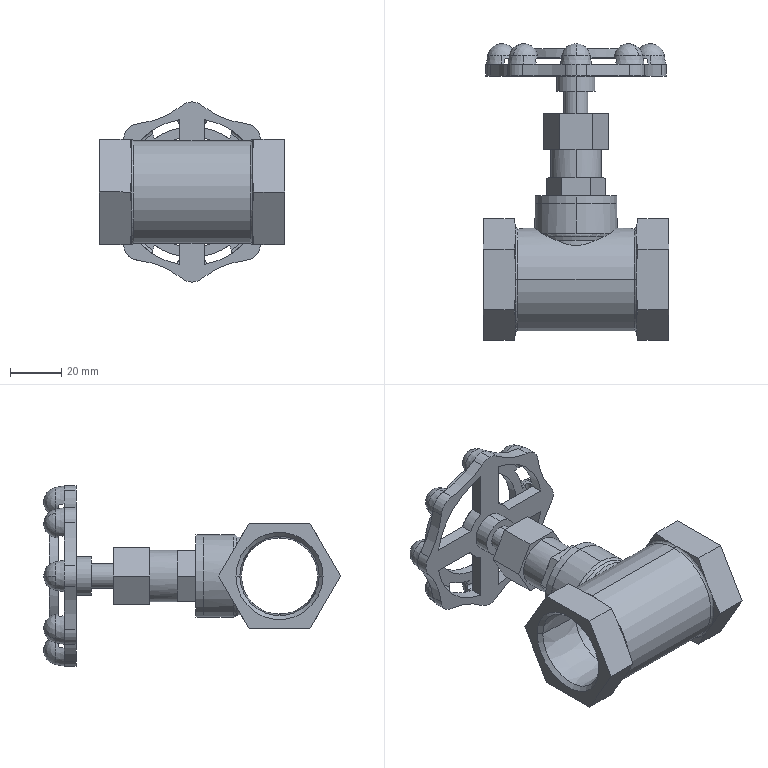Part | SolidWorks | features BaseBody 1 | 1 solid | 212 faces | box 72 x 115.407 x 70 mm | volume 83947 mm3 | plane 72 | cylinder 63 | cone 42 | torus 19 | sphere 16 | commonest cylinder face diameters 12.6 x9 23 x9 50.7 x8 66 x8 32 x4 30 x3